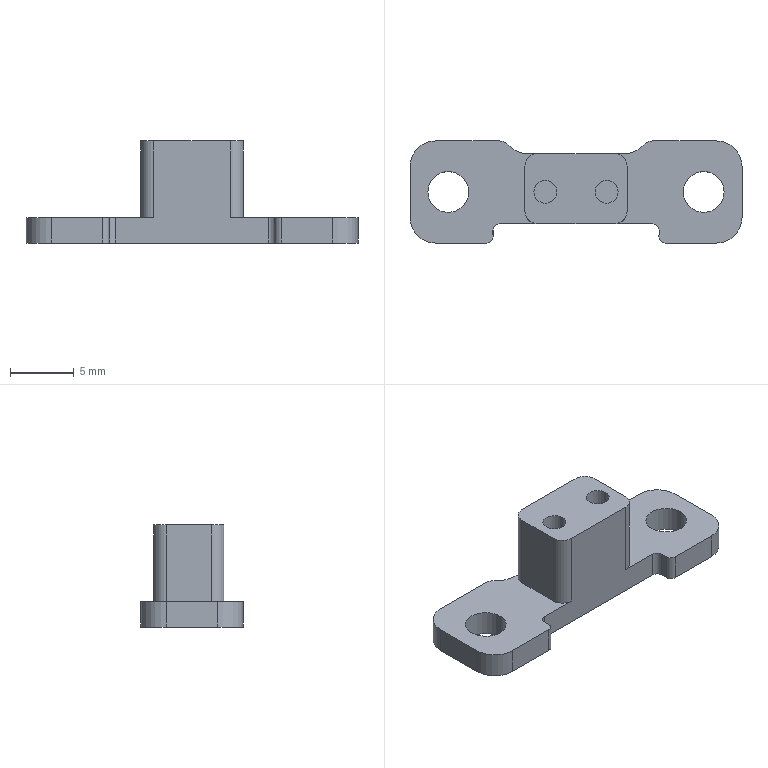NC program | Mastercam | posted with a generic post
Lines 1 to 27 of 12913:
%
:0001()
(MATERIAL - ALUMINUM MM - 2024)
(T24|100 FEM |H24)
(T8|8 FEM |H8)
(T4|4 FEM |H4)
(T1|1 FEM |H1)
(T7|4 CHM |H7)
(T6|6 FEM |H6)
N100 G21
N102 G0 G17 G40 G80 G90 G94 G98
N104 G0 G28 G91 Z0.
N106 G0 G28 X0. Y0.
(100 FEM |TOOL - 24|DIA. OFF. - 24|LEN. - 24|TOOL DIA. - 100.)
N108 T24 M6
N110 G0 G54 G90 X-100. Y0. C0. B0. S4000 M3
N112 G43 H24 Z50.
N114 Z2.
N116 G1 Z0. F600.
N118 X100. F1000.
N120 G0 Z50.
N122 M5
N124 G0 G28 G91 Z0.
N126 G28
N128 M01
N130 G0 G17 G40 G80 G90 G94 G98
N132 G0 G28 G91 Z0.